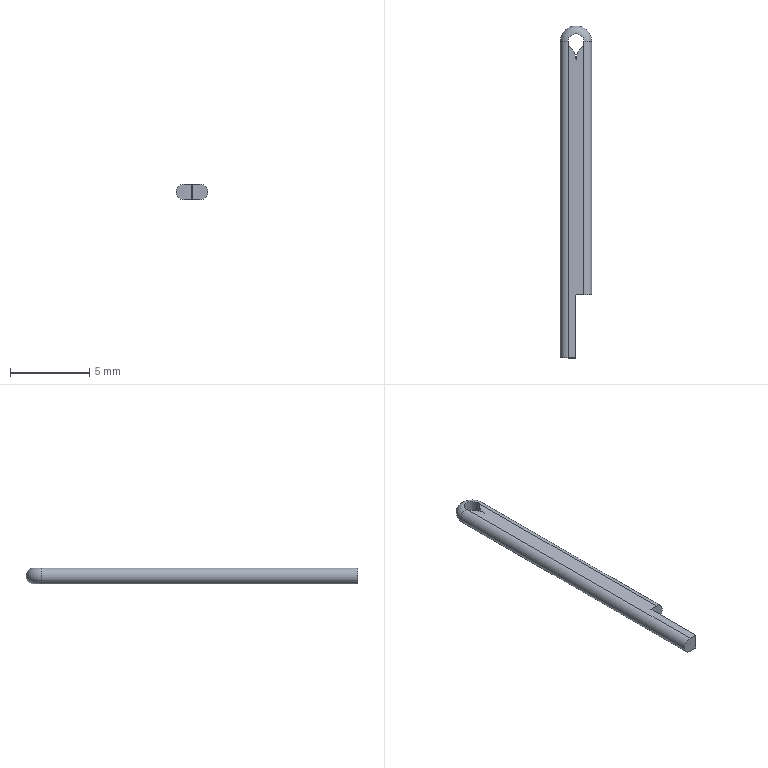Part | NX | features DATUM_CSYS 2, EXTRUDE 2, BLEND 1, SKETCH 1 | 1 solid | 11 faces | box 2 x 21 x 1 mm | volume 32.529 mm3 | plane 5 | cylinder 5 | torus 1 | commonest cylinder face diameters 1 x3 2 x2
STEP:
#1=CARTESIAN_POINT('',(1.,0.,-1.));
#2=VERTEX_POINT('',#1);
#3=CARTESIAN_POINT('',(0.5,0.,-1.));
#4=VERTEX_POINT('',#3);
#5=CARTESIAN_POINT('',(1.,0.,-1.));
#6=DIRECTION('',(-1.,0.,0.));
#7=VECTOR('',#6,1000.);
#8=LINE('',#5,#7);
#9=EDGE_CURVE('',#2,#4,#8,.T.);
#10=ORIENTED_EDGE('',*,*,#9,.T.);
#11=CARTESIAN_POINT('',(0.5,20.,-1.));
#12=VERTEX_POINT('',#11);
#13=CARTESIAN_POINT('',(0.5,20.,-1.));
#14=DIRECTION('',(0.,1.,0.));
#15=VECTOR('',#14,1000.);
#16=LINE('',#13,#15);
#17=EDGE_CURVE('',#4,#12,#16,.T.);
#18=ORIENTED_EDGE('',*,*,#17,.T.);
#19=CARTESIAN_POINT('',(0.6667,19.627,-1.));
#20=VERTEX_POINT('',#19);
#21=CARTESIAN_POINT('',(1.,20.,-1.));
#22=DIRECTION('',(0.,0.,-1.));
#23=DIRECTION('',(-1.,0.,0.));
#24=AXIS2_PLACEMENT_3D('',#21,#22,#23);
#25=CIRCLE('',#24,0.5);
#26=EDGE_CURVE('',#12,#20,#25,.F.);
#27=ORIENTED_EDGE('',*,*,#26,.T.);
#28=CARTESIAN_POINT('',(1.,18.882,-1.));
#29=VERTEX_POINT('',#28);
#30=CARTESIAN_POINT('',(0.,18.882,-1.));
#31=DIRECTION('',(0.,0.,-1.));
#32=DIRECTION('',(-1.,0.,0.));
#33=AXIS2_PLACEMENT_3D('',#30,#31,#32);
#34=CIRCLE('',#33,1.);
#35=EDGE_CURVE('',#20,#29,#34,.T.);
#36=ORIENTED_EDGE('',*,*,#35,.T.);
#37=CARTESIAN_POINT('',(1.333,19.627,-1.));
#38=VERTEX_POINT('',#37);
#39=CARTESIAN_POINT('',(2.,18.882,-1.));
#40=DIRECTION('',(0.,0.,-1.));
#41=DIRECTION('',(-1.,0.,0.));
#42=AXIS2_PLACEMENT_3D('',#39,#40,#41);
#43=CIRCLE('',#42,1.);
#44=EDGE_CURVE('',#29,#38,#43,.T.);
#45=ORIENTED_EDGE('',*,*,#44,.T.);
#46=CARTESIAN_POINT('',(1.5,20.,-1.));
#47=VERTEX_POINT('',#46);
#48=CARTESIAN_POINT('',(1.,20.,-1.));
#49=DIRECTION('',(0.,0.,-1.));
#50=DIRECTION('',(-1.,0.,0.));
#51=AXIS2_PLACEMENT_3D('',#48,#49,#50);
#52=CIRCLE('',#51,0.5);
#53=EDGE_CURVE('',#38,#47,#52,.F.);
#54=ORIENTED_EDGE('',*,*,#53,.T.);
#55=CARTESIAN_POINT('',(1.5,4.,-1.));
#56=VERTEX_POINT('',#55);
#57=CARTESIAN_POINT('',(1.5,4.,-1.));
#58=DIRECTION('',(0.,-1.,0.));
#59=VECTOR('',#58,1000.);
#60=LINE('',#57,#59);
#61=EDGE_CURVE('',#47,#56,#60,.T.);
#62=ORIENTED_EDGE('',*,*,#61,.T.);
#63=CARTESIAN_POINT('',(1.,4.,-1.));
#64=VERTEX_POINT('',#63);
#65=CARTESIAN_POINT('',(2.,4.,-1.));
#66=DIRECTION('',(-1.,0.,0.));
#67=VECTOR('',#66,1000.);
#68=LINE('',#65,#67);
#69=EDGE_CURVE('',#56,#64,#68,.T.);
#70=ORIENTED_EDGE('',*,*,#69,.T.);
#71=CARTESIAN_POINT('',(1.,4.,-1.));
#72=DIRECTION('',(0.,-1.,0.));
#73=VECTOR('',#72,1000.);
#74=LINE('',#71,#73);
#75=EDGE_CURVE('',#64,#2,#74,.T.);
#76=ORIENTED_EDGE('',*,*,#75,.T.);
#77=EDGE_LOOP('',(#10,#18,#27,#36,#45,#54,#62,#70,#76));
#78=FACE_BOUND('',#77,.T.);
#79=CARTESIAN_POINT('',(1.,20.,-1.));
#80=DIRECTION('',(0.,0.,-1.));
#81=DIRECTION('',(-1.,0.,0.));
#82=AXIS2_PLACEMENT_3D('',#79,#80,#81);
#83=PLANE('',#82);
#84=ADVANCED_FACE('',(#78),#83,.T.);
#85=CARTESIAN_POINT('',(0.6667,19.627,0.));
#86=VERTEX_POINT('',#85);
#87=CARTESIAN_POINT('',(0.5,20.,0.));
#88=VERTEX_POINT('',#87);
#89=CARTESIAN_POINT('',(1.,20.,0.));
#90=DIRECTION('',(0.,0.,-1.));
#91=DIRECTION('',(1.,0.,0.));
#92=AXIS2_PLACEMENT_3D('',#89,#90,#91);
#93=CIRCLE('',#92,0.5);
#94=EDGE_CURVE('',#86,#88,#93,.T.);
#95=ORIENTED_EDGE('',*,*,#94,.T.);
#96=CARTESIAN_POINT('',(0.5,0.,0.));
#97=VERTEX_POINT('',#96);
#98=CARTESIAN_POINT('',(0.5,20.,0.));
#99=DIRECTION('',(0.,1.,0.));
#100=VECTOR('',#99,1000.);
#101=LINE('',#98,#100);
#102=EDGE_CURVE('',#88,#97,#101,.F.);
#103=ORIENTED_EDGE('',*,*,#102,.T.);
#104=CARTESIAN_POINT('',(1.,0.,0.));
#105=VERTEX_POINT('',#104);
#106=CARTESIAN_POINT('',(1.,0.,0.));
#107=DIRECTION('',(-1.,0.,0.));
#108=VECTOR('',#107,1000.);
#109=LINE('',#106,#108);
#110=EDGE_CURVE('',#105,#97,#109,.T.);
#111=ORIENTED_EDGE('',*,*,#110,.F.);
#112=CARTESIAN_POINT('',(1.,4.,0.));
#113=VERTEX_POINT('',#112);
#114=CARTESIAN_POINT('',(1.,4.,0.));
#115=DIRECTION('',(0.,-1.,0.));
#116=VECTOR('',#115,1000.);
#117=LINE('',#114,#116);
#118=EDGE_CURVE('',#113,#105,#117,.T.);
#119=ORIENTED_EDGE('',*,*,#118,.F.);
#120=CARTESIAN_POINT('',(1.5,4.,0.));
#121=VERTEX_POINT('',#120);
#122=CARTESIAN_POINT('',(2.,4.,0.));
#123=DIRECTION('',(-1.,0.,0.));
#124=VECTOR('',#123,1000.);
#125=LINE('',#122,#124);
#126=EDGE_CURVE('',#121,#113,#125,.T.);
#127=ORIENTED_EDGE('',*,*,#126,.F.);
#128=CARTESIAN_POINT('',(1.5,20.,0.));
#129=VERTEX_POINT('',#128);
#130=CARTESIAN_POINT('',(1.5,20.,0.));
#131=DIRECTION('',(0.,-1.,0.));
#132=VECTOR('',#131,1000.);
#133=LINE('',#130,#132);
#134=EDGE_CURVE('',#121,#129,#133,.F.);
#135=ORIENTED_EDGE('',*,*,#134,.T.);
#136=CARTESIAN_POINT('',(1.333,19.627,0.));
#137=VERTEX_POINT('',#136);
#138=CARTESIAN_POINT('',(1.,20.,0.));
#139=DIRECTION('',(0.,0.,-1.));
#140=DIRECTION('',(1.,0.,0.));
#141=AXIS2_PLACEMENT_3D('',#138,#139,#140);
#142=CIRCLE('',#141,0.5);
#143=EDGE_CURVE('',#129,#137,#142,.T.);
#144=ORIENTED_EDGE('',*,*,#143,.T.);
#145=CARTESIAN_POINT('',(1.,18.882,0.));
#146=VERTEX_POINT('',#145);
#147=CARTESIAN_POINT('',(2.,18.882,0.));
#148=DIRECTION('',(0.,0.,1.));
#149=DIRECTION('',(1.,0.,0.));
#150=AXIS2_PLACEMENT_3D('',#147,#148,#149);
#151=CIRCLE('',#150,1.);
#152=EDGE_CURVE('',#137,#146,#151,.T.);
#153=ORIENTED_EDGE('',*,*,#152,.T.);
#154=CARTESIAN_POINT('',(0.,18.882,0.));
#155=DIRECTION('',(0.,0.,1.));
#156=DIRECTION('',(-1.,0.,0.));
#157=AXIS2_PLACEMENT_3D('',#154,#155,#156);
#158=CIRCLE('',#157,1.);
#159=EDGE_CURVE('',#146,#86,#158,.T.);
#160=ORIENTED_EDGE('',*,*,#159,.T.);
#161=EDGE_LOOP('',(#95,#103,#111,#119,#127,#135,#144,#153,#160));
#162=FACE_BOUND('',#161,.T.);
#163=CARTESIAN_POINT('',(1.,20.,0.));
#164=DIRECTION('',(0.,0.,-1.));
#165=DIRECTION('',(-1.,0.,0.));
#166=AXIS2_PLACEMENT_3D('',#163,#164,#165);
#167=PLANE('',#166);
#168=ADVANCED_FACE('',(#162),#167,.F.);
#169=CARTESIAN_POINT('',(0.5,0.,-0.5));
#170=DIRECTION('',(0.,1.,0.));
#171=DIRECTION('',(0.,0.,1.));
#172=AXIS2_PLACEMENT_3D('',#169,#170,#171);
#173=CIRCLE('',#172,0.5);
#174=EDGE_CURVE('',#97,#4,#173,.F.);
#175=ORIENTED_EDGE('',*,*,#174,.T.);
#176=ORIENTED_EDGE('',*,*,#9,.F.);
#177=CARTESIAN_POINT('',(1.,0.,-1.));
#178=DIRECTION('',(0.,0.,1.));
#179=VECTOR('',#178,1000.);
#180=LINE('',#177,#179);
#181=EDGE_CURVE('',#2,#105,#180,.T.);
#182=ORIENTED_EDGE('',*,*,#181,.T.);
#183=ORIENTED_EDGE('',*,*,#110,.T.);
#184=EDGE_LOOP('',(#175,#176,#182,#183));
#185=FACE_BOUND('',#184,.T.);
#186=CARTESIAN_POINT('',(1.,0.,-1.));
#187=DIRECTION('',(0.,1.,0.));
#188=DIRECTION('',(0.,0.,1.));
#189=AXIS2_PLACEMENT_3D('',#186,#187,#188);
#190=PLANE('',#189);
#191=ADVANCED_FACE('',(#185),#190,.F.);
#192=ORIENTED_EDGE('',*,*,#69,.F.);
#193=CARTESIAN_POINT('',(1.5,4.,-0.5));
#194=DIRECTION('',(0.,1.,0.));
#195=DIRECTION('',(-1.,0.,0.));
#196=AXIS2_PLACEMENT_3D('',#193,#194,#195);
#197=CIRCLE('',#196,0.5);
#198=EDGE_CURVE('',#56,#121,#197,.F.);
#199=ORIENTED_EDGE('',*,*,#198,.T.);
#200=ORIENTED_EDGE('',*,*,#126,.T.);
#201=CARTESIAN_POINT('',(1.,4.,-1.));
#202=DIRECTION('',(0.,0.,1.));
#203=VECTOR('',#202,1000.);
#204=LINE('',#201,#203);
#205=EDGE_CURVE('',#64,#113,#204,.T.);
#206=ORIENTED_EDGE('',*,*,#205,.F.);
#207=EDGE_LOOP('',(#192,#199,#200,#206));
#208=FACE_BOUND('',#207,.T.);
#209=CARTESIAN_POINT('',(2.,4.,-1.));
#210=DIRECTION('',(0.,1.,0.));
#211=DIRECTION('',(-1.,0.,0.));
#212=AXIS2_PLACEMENT_3D('',#209,#210,#211);
#213=PLANE('',#212);
#214=ADVANCED_FACE('',(#208),#213,.F.);
#215=ORIENTED_EDGE('',*,*,#118,.T.);
#216=ORIENTED_EDGE('',*,*,#181,.F.);
#217=ORIENTED_EDGE('',*,*,#75,.F.);
#218=ORIENTED_EDGE('',*,*,#205,.T.);
#219=EDGE_LOOP('',(#215,#216,#217,#218));
#220=FACE_BOUND('',#219,.T.);
#221=CARTESIAN_POINT('',(1.,4.,-1.));
#222=DIRECTION('',(-1.,0.,0.));
#223=DIRECTION('',(0.,-1.,0.));
#224=AXIS2_PLACEMENT_3D('',#221,#222,#223);
#225=PLANE('',#224);
#226=ADVANCED_FACE('',(#220),#225,.F.);
#227=CARTESIAN_POINT('',(0.6667,19.627,-2.));
#228=DIRECTION('',(0.,0.,1.));
#229=VECTOR('',#228,1000.);
#230=LINE('',#227,#229);
#231=EDGE_CURVE('',#86,#20,#230,.F.);
#232=ORIENTED_EDGE('',*,*,#231,.F.);
#233=ORIENTED_EDGE('',*,*,#159,.F.);
#234=CARTESIAN_POINT('',(1.,18.882,-2.));
#235=DIRECTION('',(0.,0.,1.));
#236=VECTOR('',#235,1000.);
#237=LINE('',#234,#236);
#238=EDGE_CURVE('',#146,#29,#237,.F.);
#239=ORIENTED_EDGE('',*,*,#238,.T.);
#240=ORIENTED_EDGE('',*,*,#35,.F.);
#241=EDGE_LOOP('',(#232,#233,#239,#240));
#242=FACE_BOUND('',#241,.T.);
#243=CARTESIAN_POINT('',(0.,18.882,-2.));
#244=DIRECTION('',(0.,0.,1.));
#245=DIRECTION('',(1.,0.,0.));
#246=AXIS2_PLACEMENT_3D('',#243,#244,#245);
#247=CYLINDRICAL_SURFACE('',#246,1.);
#248=ADVANCED_FACE('',(#242),#247,.T.);
#249=CARTESIAN_POINT('',(1.333,19.627,-2.));
#250=DIRECTION('',(0.,0.,1.));
#251=VECTOR('',#250,1000.);
#252=LINE('',#249,#251);
#253=EDGE_CURVE('',#137,#38,#252,.F.);
#254=ORIENTED_EDGE('',*,*,#253,.F.);
#255=ORIENTED_EDGE('',*,*,#143,.F.);
#256=CARTESIAN_POINT('',(1.,20.,0.));
#257=DIRECTION('',(0.,0.,-1.));
#258=DIRECTION('',(1.,0.,0.));
#259=AXIS2_PLACEMENT_3D('',#256,#257,#258);
#260=CIRCLE('',#259,0.5);
#261=EDGE_CURVE('',#88,#129,#260,.T.);
#262=ORIENTED_EDGE('',*,*,#261,.F.);
#263=ORIENTED_EDGE('',*,*,#94,.F.);
#264=ORIENTED_EDGE('',*,*,#231,.T.);
#265=ORIENTED_EDGE('',*,*,#26,.F.);
#266=CARTESIAN_POINT('',(1.,20.,-1.));
#267=DIRECTION('',(0.,0.,-1.));
#268=DIRECTION('',(-1.,0.,0.));
#269=AXIS2_PLACEMENT_3D('',#266,#267,#268);
#270=CIRCLE('',#269,0.5);
#271=EDGE_CURVE('',#47,#12,#270,.F.);
#272=ORIENTED_EDGE('',*,*,#271,.F.);
#273=ORIENTED_EDGE('',*,*,#53,.F.);
#274=EDGE_LOOP('',(#254,#255,#262,#263,#264,#265,#272,#273));
#275=FACE_BOUND('',#274,.T.);
#276=CARTESIAN_POINT('',(1.,20.,-2.));
#277=DIRECTION('',(0.,0.,1.));
#278=DIRECTION('',(1.,0.,0.));
#279=AXIS2_PLACEMENT_3D('',#276,#277,#278);
#280=CYLINDRICAL_SURFACE('',#279,0.5);
#281=ADVANCED_FACE('',(#275),#280,.F.);
#282=ORIENTED_EDGE('',*,*,#238,.F.);
#283=ORIENTED_EDGE('',*,*,#152,.F.);
#284=ORIENTED_EDGE('',*,*,#253,.T.);
#285=ORIENTED_EDGE('',*,*,#44,.F.);
#286=EDGE_LOOP('',(#282,#283,#284,#285));
#287=FACE_BOUND('',#286,.T.);
#288=CARTESIAN_POINT('',(2.,18.882,-2.));
#289=DIRECTION('',(0.,0.,1.));
#290=DIRECTION('',(1.,0.,0.));
#291=AXIS2_PLACEMENT_3D('',#288,#289,#290);
#292=CYLINDRICAL_SURFACE('',#291,1.);
#293=ADVANCED_FACE('',(#287),#292,.T.);
#294=ORIENTED_EDGE('',*,*,#134,.F.);
#295=ORIENTED_EDGE('',*,*,#198,.F.);
#296=ORIENTED_EDGE('',*,*,#61,.F.);
#297=CARTESIAN_POINT('',(1.5,20.,-0.5));
#298=DIRECTION('',(0.,1.,0.));
#299=DIRECTION('',(0.,0.,1.));
#300=AXIS2_PLACEMENT_3D('',#297,#298,#299);
#301=CIRCLE('',#300,0.5);
#302=EDGE_CURVE('',#129,#47,#301,.T.);
#303=ORIENTED_EDGE('',*,*,#302,.F.);
#304=EDGE_LOOP('',(#294,#295,#296,#303));
#305=FACE_BOUND('',#304,.T.);
#306=CARTESIAN_POINT('',(1.5,20.,-0.5));
#307=DIRECTION('',(0.,-1.,0.));
#308=DIRECTION('',(0.,0.,-1.));
#309=AXIS2_PLACEMENT_3D('',#306,#307,#308);
#310=CYLINDRICAL_SURFACE('',#309,0.5);
#311=ADVANCED_FACE('',(#305),#310,.T.);
#312=CARTESIAN_POINT('',(0.5,20.,-0.5));
#313=DIRECTION('',(0.,-1.,0.));
#314=DIRECTION('',(0.,0.,-1.));
#315=AXIS2_PLACEMENT_3D('',#312,#313,#314);
#316=CIRCLE('',#315,0.5);
#317=EDGE_CURVE('',#88,#12,#316,.T.);
#318=ORIENTED_EDGE('',*,*,#317,.F.);
#319=ORIENTED_EDGE('',*,*,#261,.T.);
#320=ORIENTED_EDGE('',*,*,#302,.T.);
#321=ORIENTED_EDGE('',*,*,#271,.T.);
#322=EDGE_LOOP('',(#318,#319,#320,#321));
#323=FACE_BOUND('',#322,.T.);
#324=CARTESIAN_POINT('',(1.,20.,-0.5));
#325=DIRECTION('',(0.,0.,-1.));
#326=DIRECTION('',(-1.,0.,0.));
#327=AXIS2_PLACEMENT_3D('',#324,#325,#326);
#328=TOROIDAL_SURFACE('',#327,0.5,0.5);
#329=ADVANCED_FACE('',(#323),#328,.T.);
#330=ORIENTED_EDGE('',*,*,#102,.F.);
#331=ORIENTED_EDGE('',*,*,#317,.T.);
#332=ORIENTED_EDGE('',*,*,#17,.F.);
#333=ORIENTED_EDGE('',*,*,#174,.F.);
#334=EDGE_LOOP('',(#330,#331,#332,#333));
#335=FACE_BOUND('',#334,.T.);
#336=CARTESIAN_POINT('',(0.5,0.,-0.5));
#337=DIRECTION('',(0.,1.,0.));
#338=DIRECTION('',(0.,0.,1.));
#339=AXIS2_PLACEMENT_3D('',#336,#337,#338);
#340=CYLINDRICAL_SURFACE('',#339,0.5);
#341=ADVANCED_FACE('',(#335),#340,.T.);
#342=CLOSED_SHELL('',(#84,#168,#191,#214,#226,#248,#281,#293,#311,#329,#341));
#343=MANIFOLD_SOLID_BREP('',#342);
#344=(LENGTH_UNIT()NAMED_UNIT(*)SI_UNIT(.MILLI.,.METRE.));
#345=UNCERTAINTY_MEASURE_WITH_UNIT(LENGTH_MEASURE(0.00001),#344,'','');
#346=(NAMED_UNIT(*)PLANE_ANGLE_UNIT()SI_UNIT($,.RADIAN.));
#347=(NAMED_UNIT(*)SI_UNIT($,.STERADIAN.)SOLID_ANGLE_UNIT());
#348=(GEOMETRIC_REPRESENTATION_CONTEXT(3)GLOBAL_UNCERTAINTY_ASSIGNED_CONTEXT((#345))GLOBAL_UNIT_ASSIGNED_CONTEXT((#344,#346,#347))REPRESENTATION_CONTEXT('',''));
#349=ADVANCED_BREP_SHAPE_REPRESENTATION('',(#343),#348);